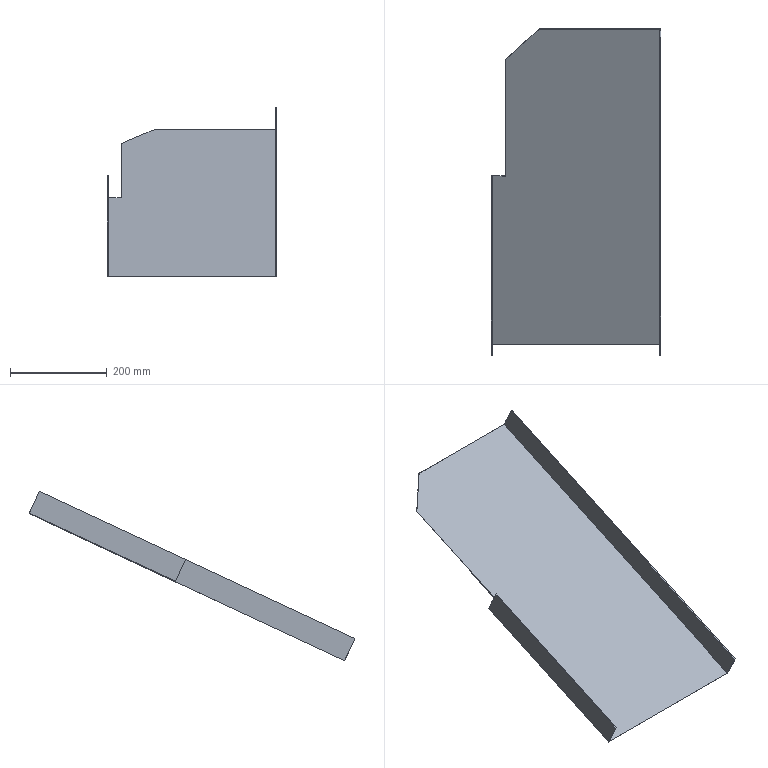Part | NX | features solid 2 | 1 solid | 14 faces | box 350 x 674.707 x 350.792 mm | volume 350900 mm3 | plane 13 | spline 1
STEP:
#1=CARTESIAN_POINT('',(562.,-1102.315,-269.141));
#2=VERTEX_POINT('',#1);
#3=CARTESIAN_POINT('',(562.,-752.431,-105.987));
#4=VERTEX_POINT('',#3);
#5=CARTESIAN_POINT('',(562.,-630.423,-49.094));
#6=DIRECTION('',(0.,-0.9063,-0.4226));
#7=VECTOR('',#6,1000.);
#8=LINE('',#5,#7);
#9=EDGE_CURVE('',#2,#4,#8,.F.);
#10=ORIENTED_EDGE('',*,*,#9,.F.);
#11=CARTESIAN_POINT('',(908.,-1102.315,-269.141));
#12=VERTEX_POINT('',#11);
#13=CARTESIAN_POINT('',(-1100.,-1102.315,-269.141));
#14=DIRECTION('',(1.,0.,0.));
#15=VECTOR('',#14,1000.);
#16=LINE('',#13,#15);
#17=EDGE_CURVE('',#12,#2,#16,.F.);
#18=ORIENTED_EDGE('',*,*,#17,.F.);
#19=CARTESIAN_POINT('',(908.,-449.161,35.43));
#20=VERTEX_POINT('',#19);
#21=CARTESIAN_POINT('',(908.,-630.423,-49.094));
#22=DIRECTION('',(0.,-0.9063,-0.4226));
#23=VECTOR('',#22,1000.);
#24=LINE('',#21,#23);
#25=EDGE_CURVE('',#12,#20,#24,.F.);
#26=ORIENTED_EDGE('',*,*,#25,.T.);
#27=CARTESIAN_POINT('',(658.755,-449.161,35.43));
#28=VERTEX_POINT('',#27);
#29=CARTESIAN_POINT('',(-1100.,-449.161,35.43));
#30=DIRECTION('',(1.,0.,0.));
#31=VECTOR('',#30,1000.);
#32=LINE('',#29,#31);
#33=EDGE_CURVE('',#20,#28,#32,.F.);
#34=ORIENTED_EDGE('',*,*,#33,.T.);
#35=CARTESIAN_POINT('',(588.755,-512.603,5.847));
#36=VERTEX_POINT('',#35);
#37=CARTESIAN_POINT('',(-320.623,-1336.778,-378.473));
#38=DIRECTION('',(0.7071,0.6409,0.2988));
#39=VECTOR('',#38,1000.);
#40=LINE('',#37,#39);
#41=EDGE_CURVE('',#28,#36,#40,.F.);
#42=ORIENTED_EDGE('',*,*,#41,.T.);
#43=CARTESIAN_POINT('',(588.755,-753.165,-106.33));
#44=VERTEX_POINT('',#43);
#45=CARTESIAN_POINT('',(588.755,-630.423,-49.094));
#46=DIRECTION('',(0.,0.9063,0.4226));
#47=VECTOR('',#46,1000.);
#48=LINE('',#45,#47);
#49=EDGE_CURVE('',#36,#44,#48,.F.);
#50=ORIENTED_EDGE('',*,*,#49,.T.);
#51=CARTESIAN_POINT('',(588.755,-753.165,-106.33));
#52=CARTESIAN_POINT('',(586.069,-753.101,-106.299));
#53=CARTESIAN_POINT('',(580.978,-752.975,-106.241));
#54=CARTESIAN_POINT('',(575.294,-752.823,-106.17));
#55=CARTESIAN_POINT('',(571.708,-752.722,-106.123));
#56=CARTESIAN_POINT('',(569.721,-752.664,-106.096));
#57=CARTESIAN_POINT('',(567.96,-752.612,-106.071));
#58=CARTESIAN_POINT('',(565.444,-752.536,-106.036));
#59=CARTESIAN_POINT('',(563.193,-752.468,-106.004));
#60=CARTESIAN_POINT('',(562.,-752.431,-105.987));
#61=B_SPLINE_CURVE_WITH_KNOTS('',3,(#51,#52,#53,#54,#55,#56,#57,#58,#59,#60),.UNSPECIFIED.,.F.,.F.,(4,1,1,1,1,1,1,4),(0.,0.02564,0.05128,0.0641,0.0705,0.07691,0.08973,0.1026),.UNSPECIFIED.);
#62=EDGE_CURVE('',#44,#4,#61,.T.);
#63=ORIENTED_EDGE('',*,*,#62,.T.);
#64=EDGE_LOOP('',(#10,#18,#26,#34,#42,#50,#63));
#65=FACE_BOUND('',#64,.T.);
#66=CARTESIAN_POINT('',(-1100.,-630.423,-49.094));
#67=DIRECTION('',(0.,0.4226,-0.9063));
#68=DIRECTION('',(0.,0.9063,0.4226));
#69=AXIS2_PLACEMENT_3D('',#66,#67,#68);
#70=PLANE('',#69);
#71=ADVANCED_FACE('',(#65),#70,.F.);
#72=ORIENTED_EDGE('',*,*,#49,.F.);
#73=CARTESIAN_POINT('',(588.755,-512.18,4.94));
#74=VERTEX_POINT('',#73);
#75=CARTESIAN_POINT('',(588.755,-512.18,4.94));
#76=DIRECTION('',(0.,0.4226,-0.9063));
#77=VECTOR('',#76,1000.);
#78=LINE('',#75,#77);
#79=EDGE_CURVE('',#36,#74,#78,.T.);
#80=ORIENTED_EDGE('',*,*,#79,.T.);
#81=CARTESIAN_POINT('',(588.755,-752.743,-107.236));
#82=VERTEX_POINT('',#81);
#83=CARTESIAN_POINT('',(588.755,-630.,-50.));
#84=DIRECTION('',(0.,0.9063,0.4226));
#85=VECTOR('',#84,1000.);
#86=LINE('',#83,#85);
#87=EDGE_CURVE('',#74,#82,#86,.F.);
#88=ORIENTED_EDGE('',*,*,#87,.T.);
#89=CARTESIAN_POINT('',(588.755,-753.165,-106.33));
#90=CARTESIAN_POINT('',(588.755,-753.024,-106.632));
#91=CARTESIAN_POINT('',(588.755,-752.883,-106.934));
#92=CARTESIAN_POINT('',(588.755,-752.743,-107.236));
#93=B_SPLINE_CURVE_WITH_KNOTS('',3,(#89,#90,#91,#92),.UNSPECIFIED.,.F.,.F.,(4,4),(0.,1.),.UNSPECIFIED.);
#94=EDGE_CURVE('',#82,#44,#93,.F.);
#95=ORIENTED_EDGE('',*,*,#94,.T.);
#96=EDGE_LOOP('',(#72,#80,#88,#95));
#97=FACE_BOUND('',#96,.T.);
#98=CARTESIAN_POINT('',(588.755,-630.,-50.));
#99=DIRECTION('',(-1.,0.,0.));
#100=DIRECTION('',(0.,0.,1.));
#101=AXIS2_PLACEMENT_3D('',#98,#99,#100);
#102=PLANE('',#101);
#103=ADVANCED_FACE('',(#97),#102,.T.);
#104=CARTESIAN_POINT('',(562.,-752.009,-106.894));
#105=VERTEX_POINT('',#104);
#106=CARTESIAN_POINT('',(562.,-752.22,-106.44));
#107=DIRECTION('',(0.,-0.4226,0.9063));
#108=VECTOR('',#107,1000.);
#109=LINE('',#106,#108);
#110=EDGE_CURVE('',#4,#105,#109,.F.);
#111=ORIENTED_EDGE('',*,*,#110,.F.);
#112=ORIENTED_EDGE('',*,*,#62,.F.);
#113=ORIENTED_EDGE('',*,*,#94,.F.);
#114=CARTESIAN_POINT('',(588.755,-752.743,-107.236));
#115=CARTESIAN_POINT('',(586.069,-752.678,-107.206));
#116=CARTESIAN_POINT('',(580.978,-752.552,-107.147));
#117=CARTESIAN_POINT('',(575.294,-752.401,-107.076));
#118=CARTESIAN_POINT('',(571.708,-752.3,-107.029));
#119=CARTESIAN_POINT('',(569.721,-752.242,-107.002));
#120=CARTESIAN_POINT('',(567.96,-752.189,-106.978));
#121=CARTESIAN_POINT('',(565.444,-752.114,-106.943));
#122=CARTESIAN_POINT('',(563.193,-752.045,-106.911));
#123=CARTESIAN_POINT('',(562.,-752.009,-106.894));
#124=B_SPLINE_CURVE_WITH_KNOTS('',3,(#114,#115,#116,#117,#118,#119,#120,#121,#122,#123),.UNSPECIFIED.,.F.,.F.,(4,1,1,1,1,1,1,4),(0.,0.02564,0.05128,0.0641,0.0705,0.07691,0.08973,0.1026),.UNSPECIFIED.);
#125=EDGE_CURVE('',#82,#105,#124,.T.);
#126=ORIENTED_EDGE('',*,*,#125,.T.);
#127=EDGE_LOOP('',(#111,#112,#113,#126));
#128=FACE_BOUND('',#127,.T.);
#129=CARTESIAN_POINT('',(588.755,-752.743,-107.236));
#130=CARTESIAN_POINT('',(588.755,-753.165,-106.33));
#131=CARTESIAN_POINT('',(586.069,-752.678,-107.206));
#132=CARTESIAN_POINT('',(586.069,-753.101,-106.299));
#133=CARTESIAN_POINT('',(580.978,-752.552,-107.147));
#134=CARTESIAN_POINT('',(580.978,-752.975,-106.241));
#135=CARTESIAN_POINT('',(575.294,-752.401,-107.076));
#136=CARTESIAN_POINT('',(575.294,-752.823,-106.17));
#137=CARTESIAN_POINT('',(571.708,-752.3,-107.029));
#138=CARTESIAN_POINT('',(571.708,-752.722,-106.123));
#139=CARTESIAN_POINT('',(569.721,-752.242,-107.002));
#140=CARTESIAN_POINT('',(569.721,-752.664,-106.096));
#141=CARTESIAN_POINT('',(567.96,-752.189,-106.978));
#142=CARTESIAN_POINT('',(567.96,-752.612,-106.071));
#143=CARTESIAN_POINT('',(565.444,-752.114,-106.943));
#144=CARTESIAN_POINT('',(565.444,-752.536,-106.036));
#145=CARTESIAN_POINT('',(563.193,-752.045,-106.911));
#146=CARTESIAN_POINT('',(563.193,-752.468,-106.004));
#147=CARTESIAN_POINT('',(562.,-752.009,-106.894));
#148=CARTESIAN_POINT('',(562.,-752.431,-105.987));
#149=B_SPLINE_SURFACE_WITH_KNOTS('',3,1,((#129,#130),(#131,#132),(#133,#134),(#135,#136),(#137,#138),(#139,#140),(#141,#142),(#143,#144),(#145,#146),(#147,#148)),.SURF_OF_LINEAR_EXTRUSION.,.F.,.F.,.F.,(4,1,1,1,1,1,1,4),(2,2),(0.,0.02564,0.05128,0.0641,0.0705,0.07691,0.08973,0.1026),(0.,1.),.UNSPECIFIED.);
#150=ADVANCED_FACE('',(#128),#149,.T.);
#151=ORIENTED_EDGE('',*,*,#17,.T.);
#152=CARTESIAN_POINT('',(562.,-1123.446,-223.825));
#153=VERTEX_POINT('',#152);
#154=CARTESIAN_POINT('',(562.,-1101.892,-270.047));
#155=DIRECTION('',(0.,-0.4226,0.9063));
#156=VECTOR('',#155,1000.);
#157=LINE('',#154,#156);
#158=EDGE_CURVE('',#2,#153,#157,.T.);
#159=ORIENTED_EDGE('',*,*,#158,.T.);
#160=CARTESIAN_POINT('',(560.,-1123.446,-223.825));
#161=VERTEX_POINT('',#160);
#162=CARTESIAN_POINT('',(540.,-1123.446,-223.825));
#163=DIRECTION('',(1.,0.,0.));
#164=VECTOR('',#163,1000.);
#165=LINE('',#162,#164);
#166=EDGE_CURVE('',#153,#161,#165,.F.);
#167=ORIENTED_EDGE('',*,*,#166,.T.);
#168=CARTESIAN_POINT('',(560.,-1101.892,-270.047));
#169=VERTEX_POINT('',#168);
#170=CARTESIAN_POINT('',(560.,-1101.892,-270.047));
#171=DIRECTION('',(0.,0.4226,-0.9063));
#172=VECTOR('',#171,1000.);
#173=LINE('',#170,#172);
#174=EDGE_CURVE('',#161,#169,#173,.T.);
#175=ORIENTED_EDGE('',*,*,#174,.T.);
#176=CARTESIAN_POINT('',(910.,-1101.892,-270.047));
#177=VERTEX_POINT('',#176);
#178=CARTESIAN_POINT('',(-1100.,-1101.892,-270.047));
#179=DIRECTION('',(1.,0.,0.));
#180=VECTOR('',#179,1000.);
#181=LINE('',#178,#180);
#182=EDGE_CURVE('',#177,#169,#181,.F.);
#183=ORIENTED_EDGE('',*,*,#182,.F.);
#184=CARTESIAN_POINT('',(910.,-1123.446,-223.825));
#185=VERTEX_POINT('',#184);
#186=CARTESIAN_POINT('',(910.,-1101.892,-270.047));
#187=DIRECTION('',(0.,-0.4226,0.9063));
#188=VECTOR('',#187,1000.);
#189=LINE('',#186,#188);
#190=EDGE_CURVE('',#177,#185,#189,.T.);
#191=ORIENTED_EDGE('',*,*,#190,.T.);
#192=CARTESIAN_POINT('',(908.,-1123.446,-223.825));
#193=VERTEX_POINT('',#192);
#194=CARTESIAN_POINT('',(910.,-1123.446,-223.825));
#195=DIRECTION('',(1.,0.,0.));
#196=VECTOR('',#195,1000.);
#197=LINE('',#194,#196);
#198=EDGE_CURVE('',#185,#193,#197,.F.);
#199=ORIENTED_EDGE('',*,*,#198,.T.);
#200=CARTESIAN_POINT('',(908.,-1123.446,-223.825));
#201=DIRECTION('',(0.,0.4226,-0.9063));
#202=VECTOR('',#201,1000.);
#203=LINE('',#200,#202);
#204=EDGE_CURVE('',#193,#12,#203,.T.);
#205=ORIENTED_EDGE('',*,*,#204,.T.);
#206=EDGE_LOOP('',(#151,#159,#167,#175,#183,#191,#199,#205));
#207=FACE_BOUND('',#206,.T.);
#208=CARTESIAN_POINT('',(-1100.,-1101.892,-270.047));
#209=DIRECTION('',(0.,0.9063,0.4226));
#210=DIRECTION('',(0.,-0.4226,0.9063));
#211=AXIS2_PLACEMENT_3D('',#208,#209,#210);
#212=PLANE('',#211);
#213=ADVANCED_FACE('',(#207),#212,.F.);
#214=CARTESIAN_POINT('',(910.,-448.738,34.524));
#215=VERTEX_POINT('',#214);
#216=CARTESIAN_POINT('',(910.,-470.292,80.745));
#217=VERTEX_POINT('',#216);
#218=CARTESIAN_POINT('',(910.,-448.738,34.524));
#219=DIRECTION('',(0.,-0.4226,0.9063));
#220=VECTOR('',#219,1000.);
#221=LINE('',#218,#220);
#222=EDGE_CURVE('',#215,#217,#221,.T.);
#223=ORIENTED_EDGE('',*,*,#222,.T.);
#224=CARTESIAN_POINT('',(910.,-470.292,80.745));
#225=DIRECTION('',(0.,-0.9063,-0.4226));
#226=VECTOR('',#225,1000.);
#227=LINE('',#224,#226);
#228=EDGE_CURVE('',#217,#185,#227,.T.);
#229=ORIENTED_EDGE('',*,*,#228,.T.);
#230=ORIENTED_EDGE('',*,*,#190,.F.);
#231=CARTESIAN_POINT('',(910.,-630.,-50.));
#232=DIRECTION('',(0.,0.9063,0.4226));
#233=VECTOR('',#232,1000.);
#234=LINE('',#231,#233);
#235=EDGE_CURVE('',#215,#177,#234,.F.);
#236=ORIENTED_EDGE('',*,*,#235,.F.);
#237=EDGE_LOOP('',(#223,#229,#230,#236));
#238=FACE_BOUND('',#237,.T.);
#239=CARTESIAN_POINT('',(910.,-630.,-50.));
#240=DIRECTION('',(-1.,0.,0.));
#241=DIRECTION('',(0.,0.,1.));
#242=AXIS2_PLACEMENT_3D('',#239,#240,#241);
#243=PLANE('',#242);
#244=ADVANCED_FACE('',(#238),#243,.F.);
#245=ORIENTED_EDGE('',*,*,#222,.F.);
#246=CARTESIAN_POINT('',(658.755,-448.738,34.524));
#247=VERTEX_POINT('',#246);
#248=CARTESIAN_POINT('',(-1100.,-448.738,34.524));
#249=DIRECTION('',(-1.,0.,0.));
#250=VECTOR('',#249,1000.);
#251=LINE('',#248,#250);
#252=EDGE_CURVE('',#247,#215,#251,.F.);
#253=ORIENTED_EDGE('',*,*,#252,.F.);
#254=CARTESIAN_POINT('',(658.755,-448.738,34.524));
#255=DIRECTION('',(0.,-0.4226,0.9063));
#256=VECTOR('',#255,1000.);
#257=LINE('',#254,#256);
#258=EDGE_CURVE('',#247,#28,#257,.T.);
#259=ORIENTED_EDGE('',*,*,#258,.T.);
#260=ORIENTED_EDGE('',*,*,#33,.F.);
#261=CARTESIAN_POINT('',(908.,-470.292,80.745));
#262=VERTEX_POINT('',#261);
#263=CARTESIAN_POINT('',(908.,-470.292,80.745));
#264=DIRECTION('',(0.,0.4226,-0.9063));
#265=VECTOR('',#264,1000.);
#266=LINE('',#263,#265);
#267=EDGE_CURVE('',#262,#20,#266,.T.);
#268=ORIENTED_EDGE('',*,*,#267,.F.);
#269=CARTESIAN_POINT('',(910.,-470.292,80.745));
#270=DIRECTION('',(1.,0.,0.));
#271=VECTOR('',#270,1000.);
#272=LINE('',#269,#271);
#273=EDGE_CURVE('',#217,#262,#272,.F.);
#274=ORIENTED_EDGE('',*,*,#273,.F.);
#275=EDGE_LOOP('',(#245,#253,#259,#260,#268,#274));
#276=FACE_BOUND('',#275,.T.);
#277=CARTESIAN_POINT('',(-1100.,-448.738,34.524));
#278=DIRECTION('',(0.,-0.9063,-0.4226));
#279=DIRECTION('',(0.,0.4226,-0.9063));
#280=AXIS2_PLACEMENT_3D('',#277,#278,#279);
#281=PLANE('',#280);
#282=ADVANCED_FACE('',(#276),#281,.F.);
#283=ORIENTED_EDGE('',*,*,#182,.T.);
#284=CARTESIAN_POINT('',(560.,-751.352,-106.587));
#285=VERTEX_POINT('',#284);
#286=CARTESIAN_POINT('',(560.,-630.,-50.));
#287=DIRECTION('',(0.,-0.9063,-0.4226));
#288=VECTOR('',#287,1000.);
#289=LINE('',#286,#288);
#290=EDGE_CURVE('',#169,#285,#289,.F.);
#291=ORIENTED_EDGE('',*,*,#290,.T.);
#292=CARTESIAN_POINT('',(562.,-751.352,-106.587));
#293=VERTEX_POINT('',#292);
#294=CARTESIAN_POINT('',(540.,-751.352,-106.587));
#295=DIRECTION('',(1.,0.,0.));
#296=VECTOR('',#295,1000.);
#297=LINE('',#294,#296);
#298=EDGE_CURVE('',#293,#285,#297,.F.);
#299=ORIENTED_EDGE('',*,*,#298,.F.);
#300=CARTESIAN_POINT('',(562.,-630.,-50.));
#301=DIRECTION('',(0.,-0.9063,-0.4226));
#302=VECTOR('',#301,1000.);
#303=LINE('',#300,#302);
#304=EDGE_CURVE('',#105,#293,#303,.F.);
#305=ORIENTED_EDGE('',*,*,#304,.F.);
#306=ORIENTED_EDGE('',*,*,#125,.F.);
#307=ORIENTED_EDGE('',*,*,#87,.F.);
#308=CARTESIAN_POINT('',(708.755,-403.423,55.655));
#309=DIRECTION('',(-0.7071,-0.6409,-0.2988));
#310=VECTOR('',#309,1000.);
#311=LINE('',#308,#310);
#312=EDGE_CURVE('',#74,#247,#311,.F.);
#313=ORIENTED_EDGE('',*,*,#312,.T.);
#314=ORIENTED_EDGE('',*,*,#252,.T.);
#315=ORIENTED_EDGE('',*,*,#235,.T.);
#316=EDGE_LOOP('',(#283,#291,#299,#305,#306,#307,#313,#314,#315));
#317=FACE_BOUND('',#316,.T.);
#318=CARTESIAN_POINT('',(-1100.,-630.,-50.));
#319=DIRECTION('',(0.,0.4226,-0.9063));
#320=DIRECTION('',(0.,0.9063,0.4226));
#321=AXIS2_PLACEMENT_3D('',#318,#319,#320);
#322=PLANE('',#321);
#323=ADVANCED_FACE('',(#317),#322,.T.);
#324=ORIENTED_EDGE('',*,*,#174,.F.);
#325=CARTESIAN_POINT('',(560.,-772.905,-60.365));
#326=VERTEX_POINT('',#325);
#327=CARTESIAN_POINT('',(560.,-114.924,246.456));
#328=DIRECTION('',(0.,0.9063,0.4226));
#329=VECTOR('',#328,1000.);
#330=LINE('',#327,#329);
#331=EDGE_CURVE('',#161,#326,#330,.T.);
#332=ORIENTED_EDGE('',*,*,#331,.T.);
#333=CARTESIAN_POINT('',(560.,-657.981,-306.821));
#334=DIRECTION('',(0.,-0.4226,0.9063));
#335=VECTOR('',#334,1000.);
#336=LINE('',#333,#335);
#337=EDGE_CURVE('',#326,#285,#336,.F.);
#338=ORIENTED_EDGE('',*,*,#337,.T.);
#339=ORIENTED_EDGE('',*,*,#290,.F.);
#340=EDGE_LOOP('',(#324,#332,#338,#339));
#341=FACE_BOUND('',#340,.T.);
#342=CARTESIAN_POINT('',(560.,0.,0.));
#343=DIRECTION('',(1.,0.,0.));
#344=DIRECTION('',(0.,0.,-1.));
#345=AXIS2_PLACEMENT_3D('',#342,#343,#344);
#346=PLANE('',#345);
#347=ADVANCED_FACE('',(#341),#346,.F.);
#348=ORIENTED_EDGE('',*,*,#312,.F.);
#349=ORIENTED_EDGE('',*,*,#79,.F.);
#350=ORIENTED_EDGE('',*,*,#41,.F.);
#351=ORIENTED_EDGE('',*,*,#258,.F.);
#352=EDGE_LOOP('',(#348,#349,#350,#351));
#353=FACE_BOUND('',#352,.T.);
#354=CARTESIAN_POINT('',(708.755,-403.423,55.655));
#355=DIRECTION('',(-0.7071,0.6409,0.2988));
#356=DIRECTION('',(-0.6715,-0.741,0.));
#357=AXIS2_PLACEMENT_3D('',#354,#355,#356);
#358=PLANE('',#357);
#359=ADVANCED_FACE('',(#353),#358,.T.);
#360=ORIENTED_EDGE('',*,*,#273,.T.);
#361=CARTESIAN_POINT('',(908.,-470.292,80.745));
#362=DIRECTION('',(0.,-0.9063,-0.4226));
#363=VECTOR('',#362,1000.);
#364=LINE('',#361,#363);
#365=EDGE_CURVE('',#262,#193,#364,.T.);
#366=ORIENTED_EDGE('',*,*,#365,.T.);
#367=ORIENTED_EDGE('',*,*,#198,.F.);
#368=ORIENTED_EDGE('',*,*,#228,.F.);
#369=EDGE_LOOP('',(#360,#366,#367,#368));
#370=FACE_BOUND('',#369,.T.);
#371=CARTESIAN_POINT('',(910.,-470.292,80.745));
#372=DIRECTION('',(0.,-0.4226,0.9063));
#373=DIRECTION('',(0.,-0.9063,-0.4226));
#374=AXIS2_PLACEMENT_3D('',#371,#372,#373);
#375=PLANE('',#374);
#376=ADVANCED_FACE('',(#370),#375,.T.);
#377=ORIENTED_EDGE('',*,*,#25,.F.);
#378=ORIENTED_EDGE('',*,*,#204,.F.);
#379=ORIENTED_EDGE('',*,*,#365,.F.);
#380=ORIENTED_EDGE('',*,*,#267,.T.);
#381=EDGE_LOOP('',(#377,#378,#379,#380));
#382=FACE_BOUND('',#381,.T.);
#383=CARTESIAN_POINT('',(908.,-470.292,80.745));
#384=DIRECTION('',(1.,0.,0.));
#385=DIRECTION('',(0.,0.,-1.));
#386=AXIS2_PLACEMENT_3D('',#383,#384,#385);
#387=PLANE('',#386);
#388=ADVANCED_FACE('',(#382),#387,.F.);
#389=ORIENTED_EDGE('',*,*,#298,.T.);
#390=ORIENTED_EDGE('',*,*,#337,.F.);
#391=CARTESIAN_POINT('',(562.,-772.905,-60.365));
#392=VERTEX_POINT('',#391);
#393=CARTESIAN_POINT('',(540.,-772.905,-60.365));
#394=DIRECTION('',(1.,0.,0.));
#395=VECTOR('',#394,1000.);
#396=LINE('',#393,#395);
#397=EDGE_CURVE('',#392,#326,#396,.F.);
#398=ORIENTED_EDGE('',*,*,#397,.F.);
#399=CARTESIAN_POINT('',(562.,-751.352,-106.587));
#400=DIRECTION('',(0.,0.4226,-0.9063));
#401=VECTOR('',#400,1000.);
#402=LINE('',#399,#401);
#403=EDGE_CURVE('',#293,#392,#402,.F.);
#404=ORIENTED_EDGE('',*,*,#403,.F.);
#405=EDGE_LOOP('',(#389,#390,#398,#404));
#406=FACE_BOUND('',#405,.T.);
#407=CARTESIAN_POINT('',(540.,-751.352,-106.587));
#408=DIRECTION('',(0.,0.9063,0.4226));
#409=DIRECTION('',(0.,-0.4226,0.9063));
#410=AXIS2_PLACEMENT_3D('',#407,#408,#409);
#411=PLANE('',#410);
#412=ADVANCED_FACE('',(#406),#411,.T.);
#413=ORIENTED_EDGE('',*,*,#397,.T.);
#414=ORIENTED_EDGE('',*,*,#331,.F.);
#415=ORIENTED_EDGE('',*,*,#166,.F.);
#416=CARTESIAN_POINT('',(562.,-1123.446,-223.825));
#417=DIRECTION('',(0.,0.9063,0.4226));
#418=VECTOR('',#417,1000.);
#419=LINE('',#416,#418);
#420=EDGE_CURVE('',#153,#392,#419,.T.);
#421=ORIENTED_EDGE('',*,*,#420,.T.);
#422=EDGE_LOOP('',(#413,#414,#415,#421));
#423=FACE_BOUND('',#422,.T.);
#424=CARTESIAN_POINT('',(540.,-1123.446,-223.825));
#425=DIRECTION('',(0.,0.4226,-0.9063));
#426=DIRECTION('',(0.,0.9063,0.4226));
#427=AXIS2_PLACEMENT_3D('',#424,#425,#426);
#428=PLANE('',#427);
#429=ADVANCED_FACE('',(#423),#428,.F.);
#430=ORIENTED_EDGE('',*,*,#158,.F.);
#431=ORIENTED_EDGE('',*,*,#9,.T.);
#432=ORIENTED_EDGE('',*,*,#110,.T.);
#433=ORIENTED_EDGE('',*,*,#304,.T.);
#434=ORIENTED_EDGE('',*,*,#403,.T.);
#435=ORIENTED_EDGE('',*,*,#420,.F.);
#436=EDGE_LOOP('',(#430,#431,#432,#433,#434,#435));
#437=FACE_BOUND('',#436,.T.);
#438=CARTESIAN_POINT('',(562.,-1101.892,-270.047));
#439=DIRECTION('',(1.,0.,0.));
#440=DIRECTION('',(0.,0.,-1.));
#441=AXIS2_PLACEMENT_3D('',#438,#439,#440);
#442=PLANE('',#441);
#443=ADVANCED_FACE('',(#437),#442,.T.);
#444=CLOSED_SHELL('',(#71,#103,#150,#213,#244,#282,#323,#347,#359,#376,#388,#412,#429,#443));
#445=MANIFOLD_SOLID_BREP('',#444);
#446=(LENGTH_UNIT()NAMED_UNIT(*)SI_UNIT(.MILLI.,.METRE.));
#447=UNCERTAINTY_MEASURE_WITH_UNIT(LENGTH_MEASURE(0.0508),#446,'','');
#448=(NAMED_UNIT(*)PLANE_ANGLE_UNIT()SI_UNIT($,.RADIAN.));
#449=(NAMED_UNIT(*)SI_UNIT($,.STERADIAN.)SOLID_ANGLE_UNIT());
#450=(GEOMETRIC_REPRESENTATION_CONTEXT(3)GLOBAL_UNCERTAINTY_ASSIGNED_CONTEXT((#447))GLOBAL_UNIT_ASSIGNED_CONTEXT((#446,#448,#449))REPRESENTATION_CONTEXT('',''));
#451=ADVANCED_BREP_SHAPE_REPRESENTATION('',(#445),#450);